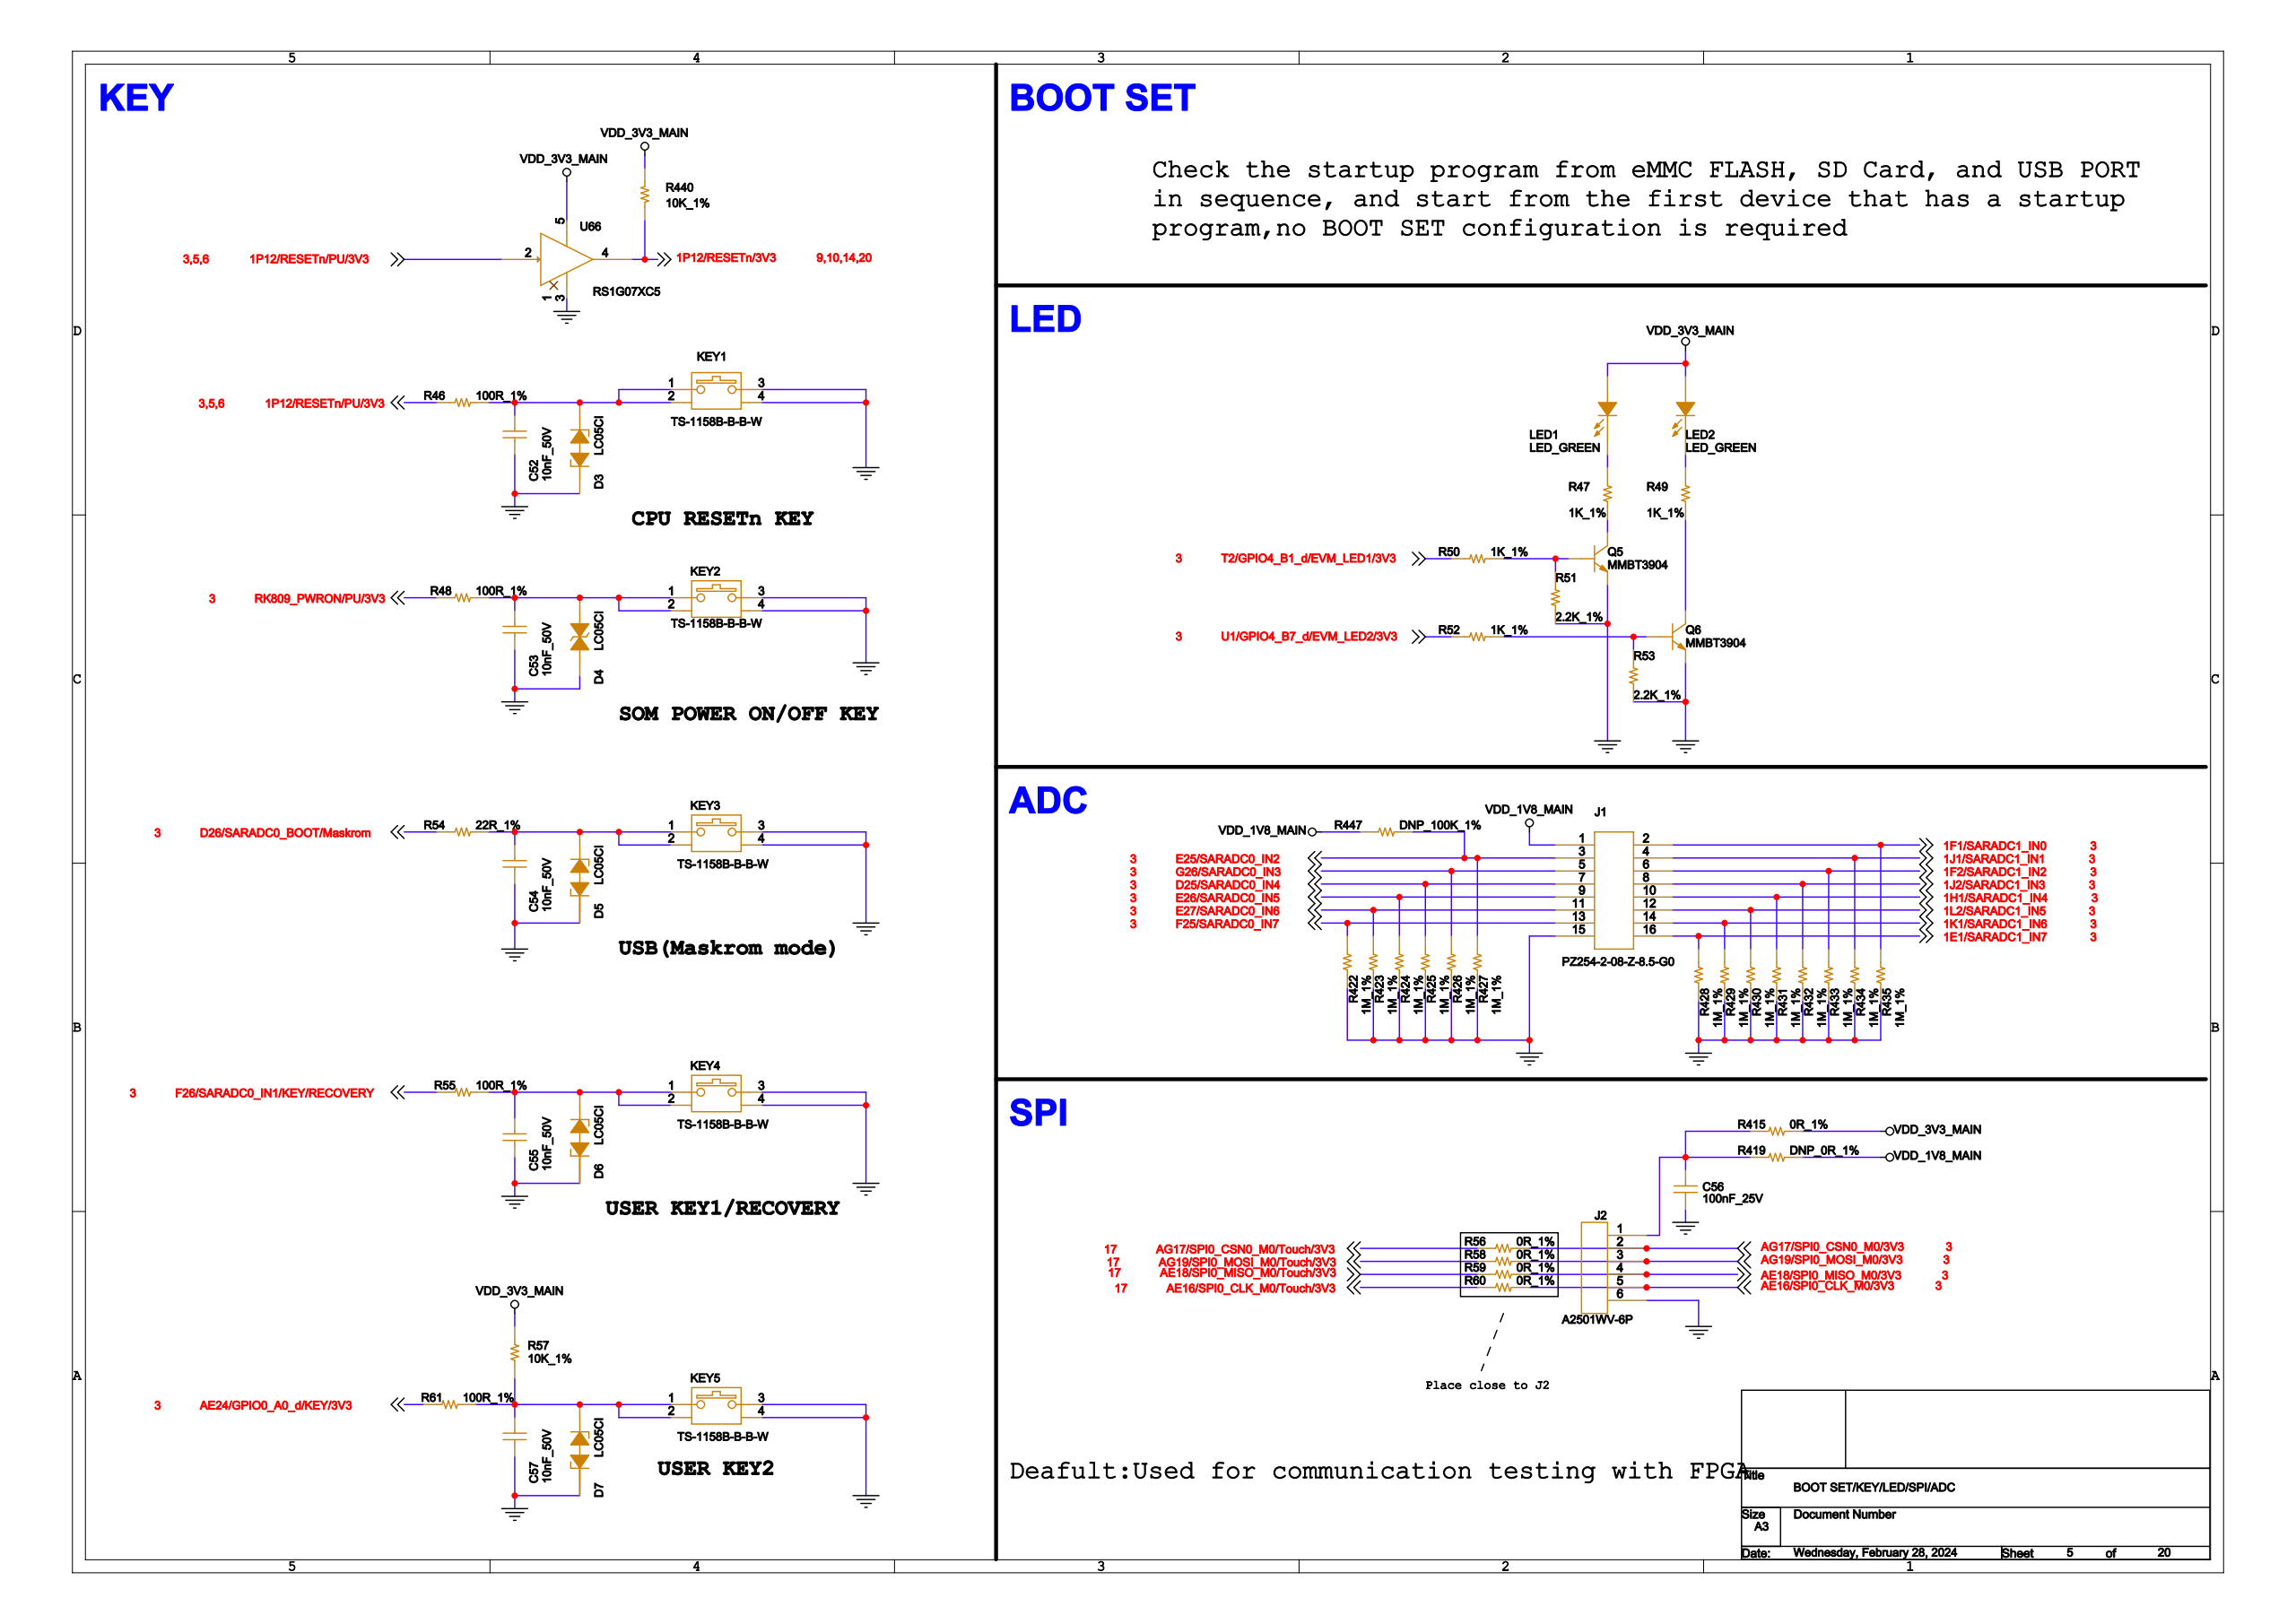Circuit board | Cadence Allegro | 1024 parts | 682 nets | one sheet of the schematic
Parts on this sheet (reference | value | footprint):
C52 | 10nF_50V | C0402
C53 | 10nF_50V | C0402
C54 | 10nF_50V | C0402
C55 | 10nF_50V | C0402
C56 | 100nF_25V | C0402
C57 | 10nF_50V | C0402
D3 | LC05CI | SOD323_BI
D4 | LC05CI | SOD323_BI
D5 | LC05CI | SOD323_BI
D6 | LC05CI | SOD323_BI
D7 | LC05CI | SOD323_BI
J1 | PZ254-2-08-Z-8.5-G0 | CON_2D54_2X8_TH
J2 | A2501WV-06A | CON_XH_1X6P_2D54_H_M_DIP
KEY1 | TS-1158B-B-B-W | TS-1158B-B-B-W
KEY2 | TS-1158B-B-B-W | TS-1158B-B-B-W
KEY3 | TS-1158B-B-B-W | TS-1158B-B-B-W
KEY4 | TS-1158B-B-B-W | TS-1158B-B-B-W
KEY5 | TS-1158B-B-B-W | TS-1158B-B-B-W
LED1 | GREEN_LED | CON_2P_3MM
LED2 | GREEN_LED | CON_2P_3MM
Q5 | MMBT3904 | SOT23-3_DBZ3
Q6 | MMBT3904 | SOT23-3_DBZ3
R46 | 100R_1% | R0603
R47 | 1K_1% | R0402
R48 | 100R_1% | R0603
R49 | 1K_1% | R0402
R50 | 1K_1% | R0402
R51 | 2.2K_1% | R0603
R52 | 1K_1% | R0402
R53 | 2.2K_1% | R0603
R54 | 22R_1% | R0402
R55 | 100R_1% | R0603
R56 | 0R_1% | R0402
R57 | 10K_1% | R0402
R58 | 0R_1% | R0402
R59 | 0R_1% | R0402
R60 | 0R_1% | R0402
R61 | 100R_1% | R0603
R415 | 0R_1% | R0603
R419 | DNP_0R_1% | R0603
R422 | 1M_1% | R0603
R423 | 1M_1% | R0603
R424 | 1M_1% | R0603
R425 | 1M_1% | R0603
R426 | 1M_1% | R0603
R427 | 1M_1% | R0603
R428 | 1M_1% | R0603
R429 | 1M_1% | R0603
R430 | 1M_1% | R0603
R431 | 1M_1% | R0603
R432 | 1M_1% | R0603
R433 | 1M_1% | R0603
R434 | 1M_1% | R0603
R435 | 1M_1% | R0603
R440 | 10K_1% | R0402
R447 | DNP_100K_1% | R0402
U66 | RS1G07XC5 | SC70-5-43M
Nets of these parts (net: part-pin ...):
GND: C52-2 C53-2 C54-2 C55-2 C56-2 C57-2 D3-2 D4-2 D5-2 D6-2 D7-2 J1-15 J2-6 KEY1-3 KEY1-4 KEY2-3 KEY2-4 KEY3-3 KEY3-4 KEY4-3 KEY4-4 KEY5-3 KEY5-4 Q5-2 Q6-2 R51-1 R53-1 R422-2 R423-2 R424-2 R425-2 R426-2 R427-2 R428-2 R429-2 R430-2 R431-2 R432-2 R433-2 R434-2 R435-2 U66-3
VDD_1V8_MAIN: J1-1 R419-2 R447-1
E25/SARADC0_IN2: J1-3 R427-1 R447-2
1H1/SARADC1_IN4: J1-10 R431-1
E27/SARADC0_IN6: J1-11 R423-1
1L2/SARADC1_IN5: J1-12 R430-1
F25/SARADC0_IN7: J1-13 R422-1
1K1/SARADC1_IN6: J1-14 R429-1
1E1/SARADC1_IN7: J1-16 R428-1
1F1/SARADC1_IN0: J1-2 R435-1
1J1/SARADC1_IN1: J1-4 R434-1
G26/SARADC0_IN3: J1-5 R426-1
1F2/SARADC1_IN2: J1-6 R433-1
D25/SARADC0_IN4: J1-7 R425-1
1J2/SARADC1_IN3: J1-8 R432-1
E26/SARADC0_IN5: J1-9 R424-1
1P12/RESETN/PU/3V3: R46-1 U66-2
VDD_3V3_MAIN: LED1-1 LED2-1 R57-2 R415-2 R440-2 U66-5
1P12/RESETN/3V3: R440-1 U66-4
N21597475: C52-1 D3-1 KEY1-1 KEY1-2 R46-2
N21597552: C53-1 D4-1 KEY2-1 KEY2-2 R48-2
N21595779: C54-1 D5-1 KEY3-1 KEY3-2 R54-2
N21598149: C55-1 D6-1 KEY4-1 KEY4-2 R55-2
N21598490: C57-1 D7-1 KEY5-1 KEY5-2 R57-1 R61-2
AG17/SPI0_CSN0_M0/3V3: J2-2 R56-2
AG19/SPI0_MOSI_M0/3V3: J2-3 R58-2
AE18/SPI0_MISO_M0/3V3: J2-4 R59-2
AE16/SPI0_CLK_M0/3V3: J2-5 R60-2
AE24/GPIO0_A0_D/KEY/3V3: R61-1
RK809_PWRON/PU/3V3: R48-1
D26/SARADC0_BOOT/MASKROM: R54-1
F26/SARADC0_IN1/KEY/RECOVERY: R55-1
T2/GPIO4_B1_D/EVM_LED1/3V3: R50-2
U1/GPIO4_B7_D/EVM_LED2/3V3: R52-2
N21652546: C56-1 J2-1 R415-1 R419-1
N21596684: Q5-3 R47-1
N21596727: LED1-2 R47-2
N21596729: Q6-3 R49-1
N21596646: LED2-2 R49-2
N21596682: Q5-1 R50-1 R51-2
N21596648: Q6-1 R52-1 R53-2
AG17/SPI0_CSN0_M0/TOUCH/3V3: R56-1
AG19/SPI0_MOSI_M0/TOUCH/3V3: R58-1
AE18/SPI0_MISO_M0/TOUCH/3V3: R59-1
AE16/SPI0_CLK_M0/TOUCH/3V3: R60-1